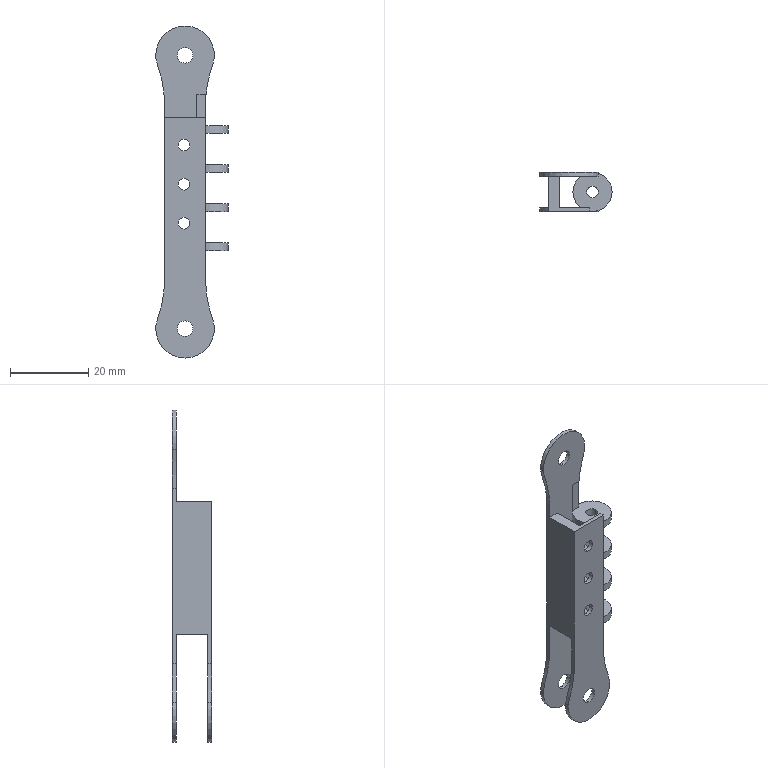Part | SolidWorks | features ICE 10, Extrusion 1 | 1 solid | 76 faces | box 18.5 x 10 x 85 mm | volume 2855 mm3 | cylinder 49 | plane 27 | commonest cylinder face diameters 3 x20 10 x12 4 x6 56.836 x6 15 x5